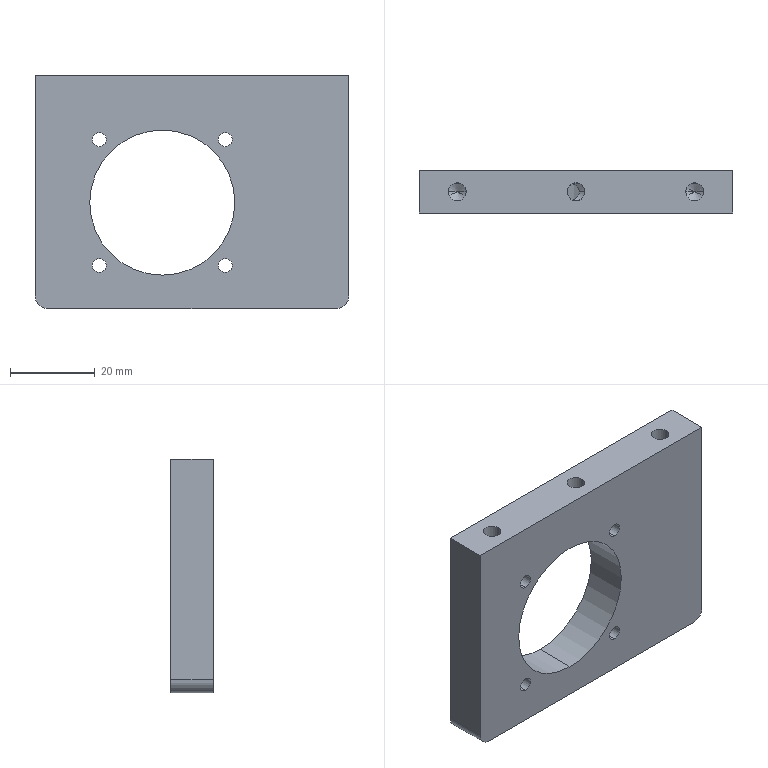Part | STEP file | PN_0009 | 1 solid | 30 faces | box 74 x 10 x 55 mm | volume 30537 mm3 | cylinder 18 | cone 6 | plane 6 | commonest cylinder face diameters 3.3 x8 4.2 x6 6 x2 34.2 x2